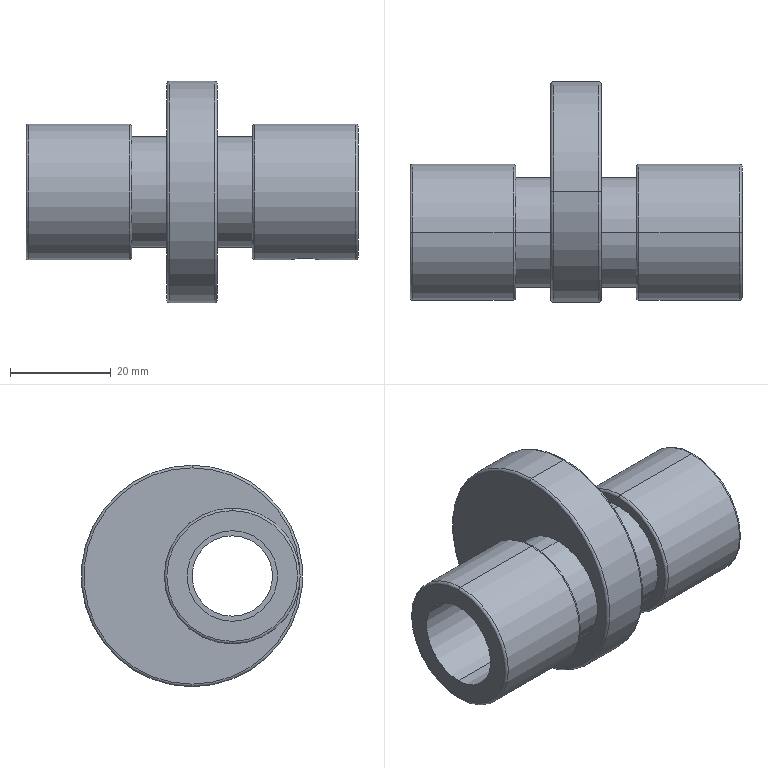Part | SolidWorks | features ICE 3, Fillet 1, Revolution 1 | 1 solid | 38 faces | box 66 x 44 x 44 mm | volume 29541 mm3 | cylinder 18 | torus 12 | plane 8 | commonest cylinder face diameters 18 x4 22 x4 27 x4 6 x2 16 x2 44 x2
STEP:
#1=CARTESIAN_POINT('',(52.5,0.,-13.5));
#2=VERTEX_POINT('',#1);
#3=CARTESIAN_POINT('',(58.5,0.,-13.5));
#4=VERTEX_POINT('',#3);
#5=CARTESIAN_POINT('',(52.5,0.,-13.5));
#6=CARTESIAN_POINT('',(52.5,-0.3922,-13.5));
#7=CARTESIAN_POINT('',(52.579,-0.7881,-13.482));
#8=CARTESIAN_POINT('',(52.804,-1.33,-13.436));
#9=CARTESIAN_POINT('',(52.898,-1.505,-13.417));
#10=CARTESIAN_POINT('',(53.116,-1.831,-13.376));
#11=CARTESIAN_POINT('',(53.239,-1.982,-13.354));
#12=CARTESIAN_POINT('',(53.516,-2.259,-13.31));
#13=CARTESIAN_POINT('',(53.67,-2.385,-13.288));
#14=CARTESIAN_POINT('',(53.994,-2.602,-13.247));
#15=CARTESIAN_POINT('',(54.166,-2.694,-13.229));
#16=CARTESIAN_POINT('',(54.712,-2.922,-13.181));
#17=CARTESIAN_POINT('',(55.103,-3.,-13.162));
#18=CARTESIAN_POINT('',(55.697,-3.,-13.162));
#19=CARTESIAN_POINT('',(55.892,-2.981,-13.167));
#20=CARTESIAN_POINT('',(56.277,-2.904,-13.184));
#21=CARTESIAN_POINT('',(56.468,-2.846,-13.197));
#22=CARTESIAN_POINT('',(56.83,-2.696,-13.228));
#23=CARTESIAN_POINT('',(57.002,-2.604,-13.247));
#24=CARTESIAN_POINT('',(57.329,-2.386,-13.288));
#25=CARTESIAN_POINT('',(57.482,-2.26,-13.31));
#26=CARTESIAN_POINT('',(57.758,-1.985,-13.354));
#27=CARTESIAN_POINT('',(57.883,-1.834,-13.376));
#28=CARTESIAN_POINT('',(58.102,-1.506,-13.417));
#29=CARTESIAN_POINT('',(58.194,-1.333,-13.435));
#30=CARTESIAN_POINT('',(58.345,-0.9726,-13.466));
#31=CARTESIAN_POINT('',(58.403,-0.7819,-13.479));
#32=CARTESIAN_POINT('',(58.48,-0.395,-13.496));
#33=CARTESIAN_POINT('',(58.5,-0.1988,-13.5));
#34=CARTESIAN_POINT('',(58.5,0.,-13.5));
#35=B_SPLINE_CURVE_WITH_KNOTS('',3,(#5,#6,#7,#8,#9,#10,#11,#12,#13,#14,#15,#16,#17,#18,#19,#20,#21,#22,#23,#24,#25,#26,#27,#28,#29,#30,#31,#32,#33,#34),.UNSPECIFIED.,.F.,.F.,(4,2,2,2,2,2,2,2,2,2,2,2,2,2,4),(0.009409,0.01058,0.01117,0.01176,0.01235,0.01294,0.01411,0.0147,0.01529,0.01588,0.01646,0.01705,0.01764,0.01823,0.01882),.UNSPECIFIED.);
#36=EDGE_CURVE('',#2,#4,#35,.T.);
#37=ORIENTED_EDGE('',*,*,#36,.F.);
#38=CARTESIAN_POINT('',(52.5,0.,-9.));
#39=VERTEX_POINT('',#38);
#40=CARTESIAN_POINT('',(52.5,0.,-26.));
#41=DIRECTION('',(0.,0.,1.));
#42=VECTOR('',#41,1000.);
#43=LINE('',#40,#42);
#44=EDGE_CURVE('',#2,#39,#43,.T.);
#45=ORIENTED_EDGE('',*,*,#44,.T.);
#46=CARTESIAN_POINT('',(58.5,0.,-9.));
#47=VERTEX_POINT('',#46);
#48=CARTESIAN_POINT('',(58.5,0.,-9.));
#49=CARTESIAN_POINT('',(58.5,-0.1998,-9.));
#50=CARTESIAN_POINT('',(58.48,-0.3959,-8.993));
#51=CARTESIAN_POINT('',(58.403,-0.7814,-8.968));
#52=CARTESIAN_POINT('',(58.345,-0.9727,-8.949));
#53=CARTESIAN_POINT('',(58.194,-1.335,-8.902));
#54=CARTESIAN_POINT('',(58.101,-1.507,-8.874));
#55=CARTESIAN_POINT('',(57.883,-1.832,-8.813));
#56=CARTESIAN_POINT('',(57.758,-1.985,-8.78));
#57=CARTESIAN_POINT('',(57.346,-2.397,-8.68));
#58=CARTESIAN_POINT('',(57.013,-2.62,-8.612));
#59=CARTESIAN_POINT('',(56.473,-2.845,-8.539));
#60=CARTESIAN_POINT('',(56.282,-2.903,-8.519));
#61=CARTESIAN_POINT('',(55.894,-2.981,-8.492));
#62=CARTESIAN_POINT('',(55.699,-3.,-8.485));
#63=CARTESIAN_POINT('',(55.304,-3.,-8.485));
#64=CARTESIAN_POINT('',(55.104,-2.98,-8.492));
#65=CARTESIAN_POINT('',(54.718,-2.903,-8.519));
#66=CARTESIAN_POINT('',(54.53,-2.846,-8.539));
#67=CARTESIAN_POINT('',(54.165,-2.694,-8.588));
#68=CARTESIAN_POINT('',(53.992,-2.601,-8.617));
#69=CARTESIAN_POINT('',(53.669,-2.384,-8.679));
#70=CARTESIAN_POINT('',(53.516,-2.259,-8.713));
#71=CARTESIAN_POINT('',(53.24,-1.982,-8.78));
#72=CARTESIAN_POINT('',(53.117,-1.832,-8.813));
#73=CARTESIAN_POINT('',(52.899,-1.508,-8.874));
#74=CARTESIAN_POINT('',(52.805,-1.333,-8.903));
#75=CARTESIAN_POINT('',(52.655,-0.9714,-8.949));
#76=CARTESIAN_POINT('',(52.598,-0.7841,-8.968));
#77=CARTESIAN_POINT('',(52.52,-0.3957,-8.993));
#78=CARTESIAN_POINT('',(52.5,-0.1968,-9.));
#79=CARTESIAN_POINT('',(52.5,0.,-9.));
#80=B_SPLINE_CURVE_WITH_KNOTS('',3,(#48,#49,#50,#51,#52,#53,#54,#55,#56,#57,#58,#59,#60,#61,#62,#63,#64,#65,#66,#67,#68,#69,#70,#71,#72,#73,#74,#75,#76,#77,#78,#79),.UNSPECIFIED.,.F.,.F.,(4,2,2,2,2,2,2,2,2,2,2,2,2,2,2,4),(0.,0.0005905,0.001181,0.001771,0.002362,0.003543,0.004133,0.004724,0.005314,0.005905,0.006495,0.007086,0.007676,0.008267,0.008857,0.009447),.UNSPECIFIED.);
#81=EDGE_CURVE('',#47,#39,#80,.T.);
#82=ORIENTED_EDGE('',*,*,#81,.F.);
#83=CARTESIAN_POINT('',(58.5,0.,-26.));
#84=DIRECTION('',(0.,0.,1.));
#85=VECTOR('',#84,1000.);
#86=LINE('',#83,#85);
#87=EDGE_CURVE('',#4,#47,#86,.T.);
#88=ORIENTED_EDGE('',*,*,#87,.F.);
#89=EDGE_LOOP('',(#37,#45,#82,#88));
#90=FACE_OUTER_BOUND('',#89,.T.);
#91=CARTESIAN_POINT('',(55.5,0.,-26.));
#92=DIRECTION('',(0.,0.,1.));
#93=DIRECTION('',(1.,0.,0.));
#94=AXIS2_PLACEMENT_3D('',#91,#92,#93);
#95=CYLINDRICAL_SURFACE('',#94,3.);
#96=ADVANCED_FACE('',(#90),#95,.F.);
#97=CARTESIAN_POINT('',(0.,0.,13.));
#98=VERTEX_POINT('',#97);
#99=CARTESIAN_POINT('',(0.,0.,-13.));
#100=VERTEX_POINT('',#99);
#101=CARTESIAN_POINT('',(0.,0.,0.));
#102=DIRECTION('',(-1.,0.,0.));
#103=DIRECTION('',(0.,0.,-1.));
#104=AXIS2_PLACEMENT_3D('',#101,#102,#103);
#105=CIRCLE('',#104,13.);
#106=EDGE_CURVE('',#98,#100,#105,.T.);
#107=ORIENTED_EDGE('',*,*,#106,.F.);
#108=CARTESIAN_POINT('',(0.5,0.,13.5));
#109=VERTEX_POINT('',#108);
#110=CARTESIAN_POINT('',(0.5,0.,13.));
#111=DIRECTION('',(0.,1.,0.));
#112=DIRECTION('',(0.,0.,1.));
#113=AXIS2_PLACEMENT_3D('',#110,#111,#112);
#114=CIRCLE('',#113,0.5);
#115=EDGE_CURVE('',#98,#109,#114,.T.);
#116=ORIENTED_EDGE('',*,*,#115,.T.);
#117=CARTESIAN_POINT('',(0.5,0.,-13.5));
#118=VERTEX_POINT('',#117);
#119=CARTESIAN_POINT('',(0.5,0.,0.));
#120=DIRECTION('',(1.,0.,0.));
#121=DIRECTION('',(0.,0.,-1.));
#122=AXIS2_PLACEMENT_3D('',#119,#120,#121);
#123=CIRCLE('',#122,13.5);
#124=EDGE_CURVE('',#118,#109,#123,.T.);
#125=ORIENTED_EDGE('',*,*,#124,.F.);
#126=CARTESIAN_POINT('',(0.5,0.,-13.));
#127=DIRECTION('',(0.,-1.,0.));
#128=DIRECTION('',(0.,0.,-1.));
#129=AXIS2_PLACEMENT_3D('',#126,#127,#128);
#130=CIRCLE('',#129,0.5);
#131=EDGE_CURVE('',#100,#118,#130,.T.);
#132=ORIENTED_EDGE('',*,*,#131,.F.);
#133=EDGE_LOOP('',(#107,#116,#125,#132));
#134=FACE_OUTER_BOUND('',#133,.T.);
#135=CARTESIAN_POINT('',(0.5,0.,0.));
#136=DIRECTION('',(1.,0.,0.));
#137=DIRECTION('',(0.,0.,-1.));
#138=AXIS2_PLACEMENT_3D('',#135,#136,#137);
#139=TOROIDAL_SURFACE('',#138,13.,0.5);
#140=ADVANCED_FACE('',(#134),#139,.T.);
#141=CARTESIAN_POINT('',(21.,0.,-13.));
#142=VERTEX_POINT('',#141);
#143=CARTESIAN_POINT('',(21.,0.,13.));
#144=VERTEX_POINT('',#143);
#145=CARTESIAN_POINT('',(21.,0.,0.));
#146=DIRECTION('',(1.,0.,0.));
#147=DIRECTION('',(0.,0.,1.));
#148=AXIS2_PLACEMENT_3D('',#145,#146,#147);
#149=CIRCLE('',#148,13.);
#150=EDGE_CURVE('',#142,#144,#149,.T.);
#151=ORIENTED_EDGE('',*,*,#150,.F.);
#152=CARTESIAN_POINT('',(20.5,0.,-13.5));
#153=VERTEX_POINT('',#152);
#154=CARTESIAN_POINT('',(20.5,0.,-13.));
#155=DIRECTION('',(0.,1.,0.));
#156=DIRECTION('',(0.,0.,1.));
#157=AXIS2_PLACEMENT_3D('',#154,#155,#156);
#158=CIRCLE('',#157,0.5);
#159=EDGE_CURVE('',#142,#153,#158,.T.);
#160=ORIENTED_EDGE('',*,*,#159,.T.);
#161=CARTESIAN_POINT('',(20.5,0.,13.5));
#162=VERTEX_POINT('',#161);
#163=CARTESIAN_POINT('',(20.5,0.,0.));
#164=DIRECTION('',(-1.,0.,0.));
#165=DIRECTION('',(0.,0.,1.));
#166=AXIS2_PLACEMENT_3D('',#163,#164,#165);
#167=CIRCLE('',#166,13.5);
#168=EDGE_CURVE('',#162,#153,#167,.T.);
#169=ORIENTED_EDGE('',*,*,#168,.F.);
#170=CARTESIAN_POINT('',(20.5,0.,13.));
#171=DIRECTION('',(0.,-1.,0.));
#172=DIRECTION('',(0.,0.,-1.));
#173=AXIS2_PLACEMENT_3D('',#170,#171,#172);
#174=CIRCLE('',#173,0.5);
#175=EDGE_CURVE('',#144,#162,#174,.T.);
#176=ORIENTED_EDGE('',*,*,#175,.F.);
#177=EDGE_LOOP('',(#151,#160,#169,#176));
#178=FACE_OUTER_BOUND('',#177,.T.);
#179=CARTESIAN_POINT('',(20.5,0.,0.));
#180=DIRECTION('',(-1.,0.,0.));
#181=DIRECTION('',(0.,0.,1.));
#182=AXIS2_PLACEMENT_3D('',#179,#180,#181);
#183=TOROIDAL_SURFACE('',#182,13.,0.5);
#184=ADVANCED_FACE('',(#178),#183,.T.);
#185=CARTESIAN_POINT('',(38.,8.,-21.5));
#186=VERTEX_POINT('',#185);
#187=CARTESIAN_POINT('',(38.,8.,21.5));
#188=VERTEX_POINT('',#187);
#189=CARTESIAN_POINT('',(38.,8.,0.));
#190=DIRECTION('',(1.,0.,0.));
#191=DIRECTION('',(0.,0.,1.));
#192=AXIS2_PLACEMENT_3D('',#189,#190,#191);
#193=CIRCLE('',#192,21.5);
#194=EDGE_CURVE('',#186,#188,#193,.T.);
#195=ORIENTED_EDGE('',*,*,#194,.F.);
#196=CARTESIAN_POINT('',(37.5,8.,-22.));
#197=VERTEX_POINT('',#196);
#198=CARTESIAN_POINT('',(37.5,8.,-21.5));
#199=DIRECTION('',(0.,1.,0.));
#200=DIRECTION('',(0.,0.,1.));
#201=AXIS2_PLACEMENT_3D('',#198,#199,#200);
#202=CIRCLE('',#201,0.5);
#203=EDGE_CURVE('',#186,#197,#202,.T.);
#204=ORIENTED_EDGE('',*,*,#203,.T.);
#205=CARTESIAN_POINT('',(37.5,8.,22.));
#206=VERTEX_POINT('',#205);
#207=CARTESIAN_POINT('',(37.5,8.,0.));
#208=DIRECTION('',(-1.,0.,0.));
#209=DIRECTION('',(0.,0.,1.));
#210=AXIS2_PLACEMENT_3D('',#207,#208,#209);
#211=CIRCLE('',#210,22.);
#212=EDGE_CURVE('',#206,#197,#211,.T.);
#213=ORIENTED_EDGE('',*,*,#212,.F.);
#214=CARTESIAN_POINT('',(37.5,8.,21.5));
#215=DIRECTION('',(0.,-1.,0.));
#216=DIRECTION('',(0.,0.,-1.));
#217=AXIS2_PLACEMENT_3D('',#214,#215,#216);
#218=CIRCLE('',#217,0.5);
#219=EDGE_CURVE('',#188,#206,#218,.T.);
#220=ORIENTED_EDGE('',*,*,#219,.F.);
#221=EDGE_LOOP('',(#195,#204,#213,#220));
#222=FACE_OUTER_BOUND('',#221,.T.);
#223=CARTESIAN_POINT('',(37.5,8.,0.));
#224=DIRECTION('',(-1.,0.,0.));
#225=DIRECTION('',(0.,0.,1.));
#226=AXIS2_PLACEMENT_3D('',#223,#224,#225);
#227=TOROIDAL_SURFACE('',#226,21.5,0.5);
#228=ADVANCED_FACE('',(#222),#227,.T.);
#229=CARTESIAN_POINT('',(28.5,8.,-22.));
#230=VERTEX_POINT('',#229);
#231=CARTESIAN_POINT('',(28.5,8.,22.));
#232=VERTEX_POINT('',#231);
#233=CARTESIAN_POINT('',(28.5,8.,0.));
#234=DIRECTION('',(1.,0.,0.));
#235=DIRECTION('',(0.,0.,1.));
#236=AXIS2_PLACEMENT_3D('',#233,#234,#235);
#237=CIRCLE('',#236,22.);
#238=EDGE_CURVE('',#230,#232,#237,.T.);
#239=ORIENTED_EDGE('',*,*,#238,.F.);
#240=CARTESIAN_POINT('',(28.,8.,-21.5));
#241=VERTEX_POINT('',#240);
#242=CARTESIAN_POINT('',(28.5,8.,-21.5));
#243=DIRECTION('',(0.,1.,0.));
#244=DIRECTION('',(0.,0.,1.));
#245=AXIS2_PLACEMENT_3D('',#242,#243,#244);
#246=CIRCLE('',#245,0.5);
#247=EDGE_CURVE('',#230,#241,#246,.T.);
#248=ORIENTED_EDGE('',*,*,#247,.T.);
#249=CARTESIAN_POINT('',(28.,8.,21.5));
#250=VERTEX_POINT('',#249);
#251=CARTESIAN_POINT('',(28.,8.,0.));
#252=DIRECTION('',(-1.,0.,0.));
#253=DIRECTION('',(0.,0.,1.));
#254=AXIS2_PLACEMENT_3D('',#251,#252,#253);
#255=CIRCLE('',#254,21.5);
#256=EDGE_CURVE('',#250,#241,#255,.T.);
#257=ORIENTED_EDGE('',*,*,#256,.F.);
#258=CARTESIAN_POINT('',(28.5,8.,21.5));
#259=DIRECTION('',(0.,-1.,0.));
#260=DIRECTION('',(0.,0.,-1.));
#261=AXIS2_PLACEMENT_3D('',#258,#259,#260);
#262=CIRCLE('',#261,0.5);
#263=EDGE_CURVE('',#232,#250,#262,.T.);
#264=ORIENTED_EDGE('',*,*,#263,.F.);
#265=EDGE_LOOP('',(#239,#248,#257,#264));
#266=FACE_OUTER_BOUND('',#265,.T.);
#267=CARTESIAN_POINT('',(28.5,8.,0.));
#268=DIRECTION('',(-1.,0.,0.));
#269=DIRECTION('',(0.,0.,1.));
#270=AXIS2_PLACEMENT_3D('',#267,#268,#269);
#271=TOROIDAL_SURFACE('',#270,21.5,0.5);
#272=ADVANCED_FACE('',(#266),#271,.T.);
#273=CARTESIAN_POINT('',(45.,0.,13.));
#274=VERTEX_POINT('',#273);
#275=CARTESIAN_POINT('',(45.,0.,-13.));
#276=VERTEX_POINT('',#275);
#277=CARTESIAN_POINT('',(45.,0.,0.));
#278=DIRECTION('',(-1.,0.,0.));
#279=DIRECTION('',(0.,0.,-1.));
#280=AXIS2_PLACEMENT_3D('',#277,#278,#279);
#281=CIRCLE('',#280,13.);
#282=EDGE_CURVE('',#274,#276,#281,.T.);
#283=ORIENTED_EDGE('',*,*,#282,.F.);
#284=CARTESIAN_POINT('',(45.5,0.,13.5));
#285=VERTEX_POINT('',#284);
#286=CARTESIAN_POINT('',(45.5,0.,13.));
#287=DIRECTION('',(0.,1.,0.));
#288=DIRECTION('',(0.,0.,1.));
#289=AXIS2_PLACEMENT_3D('',#286,#287,#288);
#290=CIRCLE('',#289,0.5);
#291=EDGE_CURVE('',#274,#285,#290,.T.);
#292=ORIENTED_EDGE('',*,*,#291,.T.);
#293=CARTESIAN_POINT('',(45.5,0.,-13.5));
#294=VERTEX_POINT('',#293);
#295=CARTESIAN_POINT('',(45.5,0.,0.));
#296=DIRECTION('',(1.,0.,0.));
#297=DIRECTION('',(0.,0.,-1.));
#298=AXIS2_PLACEMENT_3D('',#295,#296,#297);
#299=CIRCLE('',#298,13.5);
#300=EDGE_CURVE('',#294,#285,#299,.T.);
#301=ORIENTED_EDGE('',*,*,#300,.F.);
#302=CARTESIAN_POINT('',(45.5,0.,-13.));
#303=DIRECTION('',(0.,-1.,0.));
#304=DIRECTION('',(0.,0.,-1.));
#305=AXIS2_PLACEMENT_3D('',#302,#303,#304);
#306=CIRCLE('',#305,0.5);
#307=EDGE_CURVE('',#276,#294,#306,.T.);
#308=ORIENTED_EDGE('',*,*,#307,.F.);
#309=EDGE_LOOP('',(#283,#292,#301,#308));
#310=FACE_OUTER_BOUND('',#309,.T.);
#311=CARTESIAN_POINT('',(45.5,0.,0.));
#312=DIRECTION('',(1.,0.,0.));
#313=DIRECTION('',(0.,0.,-1.));
#314=AXIS2_PLACEMENT_3D('',#311,#312,#313);
#315=TOROIDAL_SURFACE('',#314,13.,0.5);
#316=ADVANCED_FACE('',(#310),#315,.T.);
#317=CARTESIAN_POINT('',(66.,0.,-13.));
#318=VERTEX_POINT('',#317);
#319=CARTESIAN_POINT('',(66.,0.,13.));
#320=VERTEX_POINT('',#319);
#321=CARTESIAN_POINT('',(66.,0.,0.));
#322=DIRECTION('',(1.,0.,0.));
#323=DIRECTION('',(0.,0.,1.));
#324=AXIS2_PLACEMENT_3D('',#321,#322,#323);
#325=CIRCLE('',#324,13.);
#326=EDGE_CURVE('',#318,#320,#325,.T.);
#327=ORIENTED_EDGE('',*,*,#326,.F.);
#328=CARTESIAN_POINT('',(65.5,0.,-13.5));
#329=VERTEX_POINT('',#328);
#330=CARTESIAN_POINT('',(65.5,0.,-13.));
#331=DIRECTION('',(0.,1.,0.));
#332=DIRECTION('',(0.,0.,1.));
#333=AXIS2_PLACEMENT_3D('',#330,#331,#332);
#334=CIRCLE('',#333,0.5);
#335=EDGE_CURVE('',#318,#329,#334,.T.);
#336=ORIENTED_EDGE('',*,*,#335,.T.);
#337=CARTESIAN_POINT('',(65.5,0.,13.5));
#338=VERTEX_POINT('',#337);
#339=CARTESIAN_POINT('',(65.5,0.,0.));
#340=DIRECTION('',(-1.,0.,0.));
#341=DIRECTION('',(0.,0.,1.));
#342=AXIS2_PLACEMENT_3D('',#339,#340,#341);
#343=CIRCLE('',#342,13.5);
#344=EDGE_CURVE('',#338,#329,#343,.T.);
#345=ORIENTED_EDGE('',*,*,#344,.F.);
#346=CARTESIAN_POINT('',(65.5,0.,13.));
#347=DIRECTION('',(0.,-1.,0.));
#348=DIRECTION('',(0.,0.,-1.));
#349=AXIS2_PLACEMENT_3D('',#346,#347,#348);
#350=CIRCLE('',#349,0.5);
#351=EDGE_CURVE('',#320,#338,#350,.T.);
#352=ORIENTED_EDGE('',*,*,#351,.F.);
#353=EDGE_LOOP('',(#327,#336,#345,#352));
#354=FACE_OUTER_BOUND('',#353,.T.);
#355=CARTESIAN_POINT('',(65.5,0.,0.));
#356=DIRECTION('',(-1.,0.,0.));
#357=DIRECTION('',(0.,0.,1.));
#358=AXIS2_PLACEMENT_3D('',#355,#356,#357);
#359=TOROIDAL_SURFACE('',#358,13.,0.5);
#360=ADVANCED_FACE('',(#354),#359,.T.);
#361=CARTESIAN_POINT('',(51.,0.,-8.));
#362=VERTEX_POINT('',#361);
#363=CARTESIAN_POINT('',(51.,0.,8.));
#364=VERTEX_POINT('',#363);
#365=CARTESIAN_POINT('',(51.,0.,0.));
#366=DIRECTION('',(-1.,0.,0.));
#367=DIRECTION('',(0.,0.,1.));
#368=AXIS2_PLACEMENT_3D('',#365,#366,#367);
#369=CIRCLE('',#368,8.);
#370=EDGE_CURVE('',#362,#364,#369,.T.);
#371=ORIENTED_EDGE('',*,*,#370,.F.);
#372=CARTESIAN_POINT('',(15.,0.,-8.));
#373=VERTEX_POINT('',#372);
#374=CARTESIAN_POINT('',(0.,0.,-8.));
#375=DIRECTION('',(-1.,0.,0.));
#376=VECTOR('',#375,1000.);
#377=LINE('',#374,#376);
#378=EDGE_CURVE('',#362,#373,#377,.T.);
#379=ORIENTED_EDGE('',*,*,#378,.T.);
#380=CARTESIAN_POINT('',(15.,0.,8.));
#381=VERTEX_POINT('',#380);
#382=CARTESIAN_POINT('',(15.,0.,0.));
#383=DIRECTION('',(-1.,0.,0.));
#384=DIRECTION('',(0.,0.,1.));
#385=AXIS2_PLACEMENT_3D('',#382,#383,#384);
#386=CIRCLE('',#385,8.);
#387=EDGE_CURVE('',#373,#381,#386,.T.);
#388=ORIENTED_EDGE('',*,*,#387,.T.);
#389=CARTESIAN_POINT('',(0.,0.,8.));
#390=DIRECTION('',(-1.,0.,0.));
#391=VECTOR('',#390,1000.);
#392=LINE('',#389,#391);
#393=EDGE_CURVE('',#364,#381,#392,.T.);
#394=ORIENTED_EDGE('',*,*,#393,.F.);
#395=EDGE_LOOP('',(#371,#379,#388,#394));
#396=FACE_OUTER_BOUND('',#395,.T.);
#397=CARTESIAN_POINT('',(0.,0.,0.));
#398=DIRECTION('',(-1.,0.,0.));
#399=DIRECTION('',(0.,0.,1.));
#400=AXIS2_PLACEMENT_3D('',#397,#398,#399);
#401=CYLINDRICAL_SURFACE('',#400,8.);
#402=ADVANCED_FACE('',(#396),#401,.F.);
#403=CARTESIAN_POINT('',(15.,0.,-9.));
#404=VERTEX_POINT('',#403);
#405=CARTESIAN_POINT('',(15.,0.,9.));
#406=VERTEX_POINT('',#405);
#407=CARTESIAN_POINT('',(15.,0.,0.));
#408=DIRECTION('',(-1.,0.,0.));
#409=DIRECTION('',(0.,0.,1.));
#410=AXIS2_PLACEMENT_3D('',#407,#408,#409);
#411=CIRCLE('',#410,9.);
#412=EDGE_CURVE('',#404,#406,#411,.T.);
#413=ORIENTED_EDGE('',*,*,#412,.F.);
#414=CARTESIAN_POINT('',(0.,0.,-9.));
#415=VERTEX_POINT('',#414);
#416=CARTESIAN_POINT('',(0.,0.,-9.));
#417=DIRECTION('',(-1.,0.,0.));
#418=VECTOR('',#417,1000.);
#419=LINE('',#416,#418);
#420=EDGE_CURVE('',#404,#415,#419,.T.);
#421=ORIENTED_EDGE('',*,*,#420,.T.);
#422=CARTESIAN_POINT('',(0.,0.,9.));
#423=VERTEX_POINT('',#422);
#424=CARTESIAN_POINT('',(0.,0.,0.));
#425=DIRECTION('',(-1.,0.,0.));
#426=DIRECTION('',(0.,0.,1.));
#427=AXIS2_PLACEMENT_3D('',#424,#425,#426);
#428=CIRCLE('',#427,9.);
#429=EDGE_CURVE('',#415,#423,#428,.T.);
#430=ORIENTED_EDGE('',*,*,#429,.T.);
#431=CARTESIAN_POINT('',(0.,0.,9.));
#432=DIRECTION('',(-1.,0.,0.));
#433=VECTOR('',#432,1000.);
#434=LINE('',#431,#433);
#435=EDGE_CURVE('',#406,#423,#434,.T.);
#436=ORIENTED_EDGE('',*,*,#435,.F.);
#437=EDGE_LOOP('',(#413,#421,#430,#436));
#438=FACE_OUTER_BOUND('',#437,.T.);
#439=CARTESIAN_POINT('',(0.,0.,0.));
#440=DIRECTION('',(-1.,0.,0.));
#441=DIRECTION('',(0.,0.,1.));
#442=AXIS2_PLACEMENT_3D('',#439,#440,#441);
#443=CYLINDRICAL_SURFACE('',#442,9.);
#444=ADVANCED_FACE('',(#438),#443,.F.);
#445=CARTESIAN_POINT('',(28.,0.,11.));
#446=VERTEX_POINT('',#445);
#447=CARTESIAN_POINT('',(28.,0.,-11.));
#448=VERTEX_POINT('',#447);
#449=CARTESIAN_POINT('',(28.,0.,0.));
#450=DIRECTION('',(-1.,0.,0.));
#451=DIRECTION('',(0.,0.,1.));
#452=AXIS2_PLACEMENT_3D('',#449,#450,#451);
#453=CIRCLE('',#452,11.);
#454=EDGE_CURVE('',#446,#448,#453,.T.);
#455=ORIENTED_EDGE('',*,*,#454,.T.);
#456=CARTESIAN_POINT('',(21.,0.,-11.));
#457=VERTEX_POINT('',#456);
#458=CARTESIAN_POINT('',(0.,0.,-11.));
#459=DIRECTION('',(-1.,0.,0.));
#460=VECTOR('',#459,1000.);
#461=LINE('',#458,#460);
#462=EDGE_CURVE('',#448,#457,#461,.T.);
#463=ORIENTED_EDGE('',*,*,#462,.T.);
#464=CARTESIAN_POINT('',(21.,0.,11.));
#465=VERTEX_POINT('',#464);
#466=CARTESIAN_POINT('',(21.,0.,0.));
#467=DIRECTION('',(-1.,0.,0.));
#468=DIRECTION('',(0.,0.,1.));
#469=AXIS2_PLACEMENT_3D('',#466,#467,#468);
#470=CIRCLE('',#469,11.);
#471=EDGE_CURVE('',#465,#457,#470,.T.);
#472=ORIENTED_EDGE('',*,*,#471,.F.);
#473=CARTESIAN_POINT('',(0.,0.,11.));
#474=DIRECTION('',(-1.,0.,0.));
#475=VECTOR('',#474,1000.);
#476=LINE('',#473,#475);
#477=EDGE_CURVE('',#446,#465,#476,.T.);
#478=ORIENTED_EDGE('',*,*,#477,.F.);
#479=EDGE_LOOP('',(#455,#463,#472,#478));
#480=FACE_OUTER_BOUND('',#479,.T.);
#481=CARTESIAN_POINT('',(0.,0.,0.));
#482=DIRECTION('',(-1.,0.,0.));
#483=DIRECTION('',(0.,0.,1.));
#484=AXIS2_PLACEMENT_3D('',#481,#482,#483);
#485=CYLINDRICAL_SURFACE('',#484,11.);
#486=ADVANCED_FACE('',(#480),#485,.T.);
#487=ORIENTED_EDGE('',*,*,#168,.T.);
#488=CARTESIAN_POINT('',(0.,0.,-13.5));
#489=DIRECTION('',(-1.,0.,0.));
#490=VECTOR('',#489,1000.);
#491=LINE('',#488,#490);
#492=EDGE_CURVE('',#153,#118,#491,.T.);
#493=ORIENTED_EDGE('',*,*,#492,.T.);
#494=ORIENTED_EDGE('',*,*,#124,.T.);
#495=CARTESIAN_POINT('',(0.,0.,13.5));
#496=DIRECTION('',(-1.,0.,0.));
#497=VECTOR('',#496,1000.);
#498=LINE('',#495,#497);
#499=EDGE_CURVE('',#162,#109,#498,.T.);
#500=ORIENTED_EDGE('',*,*,#499,.F.);
#501=EDGE_LOOP('',(#487,#493,#494,#500));
#502=FACE_OUTER_BOUND('',#501,.T.);
#503=CARTESIAN_POINT('',(0.,0.,0.));
#504=DIRECTION('',(-1.,0.,0.));
#505=DIRECTION('',(0.,0.,1.));
#506=AXIS2_PLACEMENT_3D('',#503,#504,#505);
#507=CYLINDRICAL_SURFACE('',#506,13.5);
#508=ADVANCED_FACE('',(#502),#507,.T.);
#509=ORIENTED_EDGE('',*,*,#212,.T.);
#510=CARTESIAN_POINT('',(38.,8.,-22.));
#511=DIRECTION('',(-1.,0.,0.));
#512=VECTOR('',#511,1000.);
#513=LINE('',#510,#512);
#514=EDGE_CURVE('',#197,#230,#513,.T.);
#515=ORIENTED_EDGE('',*,*,#514,.T.);
#516=ORIENTED_EDGE('',*,*,#238,.T.);
#517=CARTESIAN_POINT('',(38.,8.,22.));
#518=DIRECTION('',(-1.,0.,0.));
#519=VECTOR('',#518,1000.);
#520=LINE('',#517,#519);
#521=EDGE_CURVE('',#206,#232,#520,.T.);
#522=ORIENTED_EDGE('',*,*,#521,.F.);
#523=EDGE_LOOP('',(#509,#515,#516,#522));
#524=FACE_OUTER_BOUND('',#523,.T.);
#525=CARTESIAN_POINT('',(38.,8.,0.));
#526=DIRECTION('',(-1.,0.,0.));
#527=DIRECTION('',(0.,0.,1.));
#528=AXIS2_PLACEMENT_3D('',#525,#526,#527);
#529=CYLINDRICAL_SURFACE('',#528,22.);
#530=ADVANCED_FACE('',(#524),#529,.T.);
#531=CARTESIAN_POINT('',(66.,0.,-9.));
#532=VERTEX_POINT('',#531);
#533=CARTESIAN_POINT('',(66.,0.,9.));
#534=VERTEX_POINT('',#533);
#535=CARTESIAN_POINT('',(66.,0.,0.));
#536=DIRECTION('',(-1.,0.,0.));
#537=DIRECTION('',(0.,0.,1.));
#538=AXIS2_PLACEMENT_3D('',#535,#536,#537);
#539=CIRCLE('',#538,9.);
#540=EDGE_CURVE('',#532,#534,#539,.T.);
#541=ORIENTED_EDGE('',*,*,#540,.F.);
#542=CARTESIAN_POINT('',(0.,0.,-9.));
#543=DIRECTION('',(-1.,0.,0.));
#544=VECTOR('',#543,1000.);
#545=LINE('',#542,#544);
#546=EDGE_CURVE('',#532,#47,#545,.T.);
#547=ORIENTED_EDGE('',*,*,#546,.T.);
#548=ORIENTED_EDGE('',*,*,#81,.T.);
#549=CARTESIAN_POINT('',(51.,0.,-9.));
#550=VERTEX_POINT('',#549);
#551=CARTESIAN_POINT('',(0.,0.,-9.));
#552=DIRECTION('',(-1.,0.,0.));
#553=VECTOR('',#552,1000.);
#554=LINE('',#551,#553);
#555=EDGE_CURVE('',#39,#550,#554,.T.);
#556=ORIENTED_EDGE('',*,*,#555,.T.);
#557=CARTESIAN_POINT('',(51.,0.,9.));
#558=VERTEX_POINT('',#557);
#559=CARTESIAN_POINT('',(51.,0.,0.));
#560=DIRECTION('',(-1.,0.,0.));
#561=DIRECTION('',(0.,0.,1.));
#562=AXIS2_PLACEMENT_3D('',#559,#560,#561);
#563=CIRCLE('',#562,9.);
#564=EDGE_CURVE('',#550,#558,#563,.T.);
#565=ORIENTED_EDGE('',*,*,#564,.T.);
#566=CARTESIAN_POINT('',(0.,0.,9.));
#567=DIRECTION('',(-1.,0.,0.));
#568=VECTOR('',#567,1000.);
#569=LINE('',#566,#568);
#570=EDGE_CURVE('',#534,#558,#569,.T.);
#571=ORIENTED_EDGE('',*,*,#570,.F.);
#572=EDGE_LOOP('',(#541,#547,#548,#556,#565,#571));
#573=FACE_OUTER_BOUND('',#572,.T.);
#574=CARTESIAN_POINT('',(0.,0.,0.));
#575=DIRECTION('',(-1.,0.,0.));
#576=DIRECTION('',(0.,0.,1.));
#577=AXIS2_PLACEMENT_3D('',#574,#575,#576);
#578=CYLINDRICAL_SURFACE('',#577,9.);
#579=ADVANCED_FACE('',(#573),#578,.F.);
#580=ORIENTED_EDGE('',*,*,#344,.T.);
#581=CARTESIAN_POINT('',(0.,0.,-13.5));
#582=DIRECTION('',(-1.,0.,0.));
#583=VECTOR('',#582,1000.);
#584=LINE('',#581,#583);
#585=EDGE_CURVE('',#329,#4,#584,.T.);
#586=ORIENTED_EDGE('',*,*,#585,.T.);
#587=CARTESIAN_POINT('',(58.5,0.,-13.5));
#588=CARTESIAN_POINT('',(58.5,0.1989,-13.5));
#589=CARTESIAN_POINT('',(58.48,0.3943,-13.496));
#590=CARTESIAN_POINT('',(58.404,0.7786,-13.479));
#591=CARTESIAN_POINT('',(58.346,0.9695,-13.466));
#592=CARTESIAN_POINT('',(58.195,1.333,-13.435));
#593=CARTESIAN_POINT('',(58.103,1.505,-13.417));
#594=CARTESIAN_POINT('',(57.885,1.83,-13.376));
#595=CARTESIAN_POINT('',(57.759,1.984,-13.354));
#596=CARTESIAN_POINT('',(57.483,2.26,-13.31));
#597=CARTESIAN_POINT('',(57.332,2.384,-13.288));
#598=CARTESIAN_POINT('',(57.004,2.603,-13.247));
#599=CARTESIAN_POINT('',(56.831,2.696,-13.228));
#600=CARTESIAN_POINT('',(56.47,2.846,-13.197));
#601=CARTESIAN_POINT('',(56.28,2.903,-13.184));
#602=CARTESIAN_POINT('',(55.893,2.981,-13.167));
#603=CARTESIAN_POINT('',(55.698,3.,-13.162));
#604=CARTESIAN_POINT('',(55.305,3.,-13.162));
#605=CARTESIAN_POINT('',(55.105,2.98,-13.167));
#606=CARTESIAN_POINT('',(54.72,2.903,-13.184));
#607=CARTESIAN_POINT('',(54.533,2.847,-13.197));
#608=CARTESIAN_POINT('',(54.169,2.696,-13.228));
#609=CARTESIAN_POINT('',(53.994,2.602,-13.247));
#610=CARTESIAN_POINT('',(53.67,2.385,-13.288));
#611=CARTESIAN_POINT('',(53.518,2.26,-13.31));
#612=CARTESIAN_POINT('',(53.239,1.982,-13.354));
#613=CARTESIAN_POINT('',(53.116,1.831,-13.376));
#614=CARTESIAN_POINT('',(52.898,1.507,-13.417));
#615=CARTESIAN_POINT('',(52.804,1.331,-13.435));
#616=CARTESIAN_POINT('',(52.654,0.9683,-13.466));
#617=CARTESIAN_POINT('',(52.597,0.7813,-13.479));
#618=CARTESIAN_POINT('',(52.52,0.3953,-13.496));
#619=CARTESIAN_POINT('',(52.5,0.1961,-13.5));
#620=CARTESIAN_POINT('',(52.5,0.,-13.5));
#621=B_SPLINE_CURVE_WITH_KNOTS('',3,(#587,#588,#589,#590,#591,#592,#593,#594,#595,#596,#597,#598,#599,#600,#601,#602,#603,#604,#605,#606,#607,#608,#609,#610,#611,#612,#613,#614,#615,#616,#617,#618,#619,#620),.UNSPECIFIED.,.F.,.F.,(4,2,2,2,2,2,2,2,2,2,2,2,2,2,2,2,4),(0.,0.0005881,0.001176,0.001764,0.002352,0.00294,0.003528,0.004116,0.004704,0.005292,0.005881,0.006469,0.007057,0.007645,0.008233,0.008821,0.009409),.UNSPECIFIED.);
#622=EDGE_CURVE('',#4,#2,#621,.T.);
#623=ORIENTED_EDGE('',*,*,#622,.T.);
#624=CARTESIAN_POINT('',(0.,0.,-13.5));
#625=DIRECTION('',(-1.,0.,0.));
#626=VECTOR('',#625,1000.);
#627=LINE('',#624,#626);
#628=EDGE_CURVE('',#2,#294,#627,.T.);
#629=ORIENTED_EDGE('',*,*,#628,.T.);
#630=ORIENTED_EDGE('',*,*,#300,.T.);
#631=CARTESIAN_POINT('',(0.,0.,13.5));
#632=DIRECTION('',(-1.,0.,0.));
#633=VECTOR('',#632,1000.);
#634=LINE('',#631,#633);
#635=EDGE_CURVE('',#338,#285,#634,.T.);
#636=ORIENTED_EDGE('',*,*,#635,.F.);
#637=EDGE_LOOP('',(#580,#586,#623,#629,#630,#636));
#638=FACE_OUTER_BOUND('',#637,.T.);
#639=CARTESIAN_POINT('',(0.,0.,0.));
#640=DIRECTION('',(-1.,0.,0.));
#641=DIRECTION('',(0.,0.,1.));
#642=AXIS2_PLACEMENT_3D('',#639,#640,#641);
#643=CYLINDRICAL_SURFACE('',#642,13.5);
#644=ADVANCED_FACE('',(#638),#643,.T.);
#645=CARTESIAN_POINT('',(45.,0.,11.));
#646=VERTEX_POINT('',#645);
#647=CARTESIAN_POINT('',(45.,0.,-11.));
#648=VERTEX_POINT('',#647);
#649=CARTESIAN_POINT('',(45.,0.,0.));
#650=DIRECTION('',(-1.,0.,0.));
#651=DIRECTION('',(0.,0.,1.));
#652=AXIS2_PLACEMENT_3D('',#649,#650,#651);
#653=CIRCLE('',#652,11.);
#654=EDGE_CURVE('',#646,#648,#653,.T.);
#655=ORIENTED_EDGE('',*,*,#654,.T.);
#656=CARTESIAN_POINT('',(38.,0.,-11.));
#657=VERTEX_POINT('',#656);
#658=CARTESIAN_POINT('',(0.,0.,-11.));
#659=DIRECTION('',(-1.,0.,0.));
#660=VECTOR('',#659,1000.);
#661=LINE('',#658,#660);
#662=EDGE_CURVE('',#648,#657,#661,.T.);
#663=ORIENTED_EDGE('',*,*,#662,.T.);
#664=CARTESIAN_POINT('',(38.,0.,11.));
#665=VERTEX_POINT('',#664);
#666=CARTESIAN_POINT('',(38.,0.,0.));
#667=DIRECTION('',(-1.,0.,0.));
#668=DIRECTION('',(0.,0.,1.));
#669=AXIS2_PLACEMENT_3D('',#666,#667,#668);
#670=CIRCLE('',#669,11.);
#671=EDGE_CURVE('',#665,#657,#670,.T.);
#672=ORIENTED_EDGE('',*,*,#671,.F.);
#673=CARTESIAN_POINT('',(0.,0.,11.));
#674=DIRECTION('',(-1.,0.,0.));
#675=VECTOR('',#674,1000.);
#676=LINE('',#673,#675);
#677=EDGE_CURVE('',#646,#665,#676,.T.);
#678=ORIENTED_EDGE('',*,*,#677,.F.);
#679=EDGE_LOOP('',(#655,#663,#672,#678));
#680=FACE_OUTER_BOUND('',#679,.T.);
#681=CARTESIAN_POINT('',(0.,0.,0.));
#682=DIRECTION('',(-1.,0.,0.));
#683=DIRECTION('',(0.,0.,1.));
#684=AXIS2_PLACEMENT_3D('',#681,#682,#683);
#685=CYLINDRICAL_SURFACE('',#684,11.);
#686=ADVANCED_FACE('',(#680),#685,.T.);
#687=ORIENTED_EDGE('',*,*,#662,.F.);
#688=CARTESIAN_POINT('',(45.,0.,0.));
#689=DIRECTION('',(-1.,0.,0.));
#690=DIRECTION('',(0.,0.,1.));
#691=AXIS2_PLACEMENT_3D('',#688,#689,#690);
#692=CIRCLE('',#691,11.);
#693=EDGE_CURVE('',#648,#646,#692,.T.);
#694=ORIENTED_EDGE('',*,*,#693,.T.);
#695=ORIENTED_EDGE('',*,*,#677,.T.);
#696=CARTESIAN_POINT('',(38.,0.,0.));
#697=DIRECTION('',(-1.,0.,0.));
#698=DIRECTION('',(0.,0.,1.));
#699=AXIS2_PLACEMENT_3D('',#696,#697,#698);
#700=CIRCLE('',#699,11.);
#701=EDGE_CURVE('',#657,#665,#700,.T.);
#702=ORIENTED_EDGE('',*,*,#701,.F.);
#703=EDGE_LOOP('',(#687,#694,#695,#702));
#704=FACE_OUTER_BOUND('',#703,.T.);
#705=CARTESIAN_POINT('',(0.,0.,0.));
#706=DIRECTION('',(-1.,0.,0.));
#707=DIRECTION('',(0.,0.,1.));
#708=AXIS2_PLACEMENT_3D('',#705,#706,#707);
#709=CYLINDRICAL_SURFACE('',#708,11.);
#710=ADVANCED_FACE('',(#704),#709,.T.);
#711=CARTESIAN_POINT('',(45.,0.,0.));
#712=DIRECTION('',(-1.,0.,0.));
#713=DIRECTION('',(0.,0.,-1.));
#714=AXIS2_PLACEMENT_3D('',#711,#712,#713);
#715=CIRCLE('',#714,13.);
#716=EDGE_CURVE('',#276,#274,#715,.T.);
#717=ORIENTED_EDGE('',*,*,#716,.T.);
#718=ORIENTED_EDGE('',*,*,#282,.T.);
#719=EDGE_LOOP('',(#717,#718));
#720=FACE_OUTER_BOUND('',#719,.T.);
#721=ORIENTED_EDGE('',*,*,#654,.F.);
#722=ORIENTED_EDGE('',*,*,#693,.F.);
#723=EDGE_LOOP('',(#721,#722));
#724=FACE_BOUND('',#723,.T.);
#725=CARTESIAN_POINT('',(45.,11.,0.));
#726=DIRECTION('',(1.,0.,0.));
#727=DIRECTION('',(0.,0.,-1.));
#728=AXIS2_PLACEMENT_3D('',#725,#726,#727);
#729=PLANE('',#728);
#730=ADVANCED_FACE('',(#720,#724),#729,.F.);
#731=ORIENTED_EDGE('',*,*,#585,.F.);
#732=CARTESIAN_POINT('',(65.5,0.,0.));
#733=DIRECTION('',(-1.,0.,0.));
#734=DIRECTION('',(0.,0.,1.));
#735=AXIS2_PLACEMENT_3D('',#732,#733,#734);
#736=CIRCLE('',#735,13.5);
#737=EDGE_CURVE('',#329,#338,#736,.T.);
#738=ORIENTED_EDGE('',*,*,#737,.T.);
#739=ORIENTED_EDGE('',*,*,#635,.T.);
#740=CARTESIAN_POINT('',(45.5,0.,0.));
#741=DIRECTION('',(1.,0.,0.));
#742=DIRECTION('',(0.,0.,-1.));
#743=AXIS2_PLACEMENT_3D('',#740,#741,#742);
#744=CIRCLE('',#743,13.5);
#745=EDGE_CURVE('',#285,#294,#744,.T.);
#746=ORIENTED_EDGE('',*,*,#745,.T.);
#747=ORIENTED_EDGE('',*,*,#628,.F.);
#748=ORIENTED_EDGE('',*,*,#36,.T.);
#749=EDGE_LOOP('',(#731,#738,#739,#746,#747,#748));
#750=FACE_OUTER_BOUND('',#749,.T.);
#751=CARTESIAN_POINT('',(0.,0.,0.));
#752=DIRECTION('',(-1.,0.,0.));
#753=DIRECTION('',(0.,0.,1.));
#754=AXIS2_PLACEMENT_3D('',#751,#752,#753);
#755=CYLINDRICAL_SURFACE('',#754,13.5);
#756=ADVANCED_FACE('',(#750),#755,.T.);
#757=CARTESIAN_POINT('',(66.,0.,0.));
#758=DIRECTION('',(1.,0.,0.));
#759=DIRECTION('',(0.,0.,1.));
#760=AXIS2_PLACEMENT_3D('',#757,#758,#759);
#761=CIRCLE('',#760,13.);
#762=EDGE_CURVE('',#320,#318,#761,.T.);
#763=ORIENTED_EDGE('',*,*,#762,.T.);
#764=ORIENTED_EDGE('',*,*,#326,.T.);
#765=EDGE_LOOP('',(#763,#764));
#766=FACE_OUTER_BOUND('',#765,.T.);
#767=CARTESIAN_POINT('',(66.,0.,0.));
#768=DIRECTION('',(-1.,0.,0.));
#769=DIRECTION('',(0.,0.,1.));
#770=AXIS2_PLACEMENT_3D('',#767,#768,#769);
#771=CIRCLE('',#770,9.);
#772=EDGE_CURVE('',#534,#532,#771,.T.);
#773=ORIENTED_EDGE('',*,*,#772,.T.);
#774=ORIENTED_EDGE('',*,*,#540,.T.);
#775=EDGE_LOOP('',(#773,#774));
#776=FACE_BOUND('',#775,.T.);
#777=CARTESIAN_POINT('',(66.,13.5,0.));
#778=DIRECTION('',(-1.,0.,0.));
#779=DIRECTION('',(0.,0.,1.));
#780=AXIS2_PLACEMENT_3D('',#777,#778,#779);
#781=PLANE('',#780);
#782=ADVANCED_FACE('',(#766,#776),#781,.F.);
#783=ORIENTED_EDGE('',*,*,#546,.F.);
#784=ORIENTED_EDGE('',*,*,#772,.F.);
#785=ORIENTED_EDGE('',*,*,#570,.T.);
#786=CARTESIAN_POINT('',(51.,0.,0.));
#787=DIRECTION('',(-1.,0.,0.));
#788=DIRECTION('',(0.,0.,1.));
#789=AXIS2_PLACEMENT_3D('',#786,#787,#788);
#790=CIRCLE('',#789,9.);
#791=EDGE_CURVE('',#558,#550,#790,.T.);
#792=ORIENTED_EDGE('',*,*,#791,.T.);
#793=ORIENTED_EDGE('',*,*,#555,.F.);
#794=CARTESIAN_POINT('',(52.5,0.,-9.));
#795=CARTESIAN_POINT('',(52.5,0.1967,-9.));
#796=CARTESIAN_POINT('',(52.519,0.3948,-8.993));
#797=CARTESIAN_POINT('',(52.597,0.784,-8.968));
#798=CARTESIAN_POINT('',(52.655,0.9716,-8.949));
#799=CARTESIAN_POINT('',(52.806,1.334,-8.903));
#800=CARTESIAN_POINT('',(52.9,1.509,-8.874));
#801=CARTESIAN_POINT('',(53.117,1.833,-8.813));
#802=CARTESIAN_POINT('',(53.241,1.983,-8.78));
#803=CARTESIAN_POINT('',(53.656,2.399,-8.679));
#804=CARTESIAN_POINT('',(53.983,2.618,-8.612));
#805=CARTESIAN_POINT('',(54.53,2.846,-8.539));
#806=CARTESIAN_POINT('',(54.718,2.903,-8.519));
#807=CARTESIAN_POINT('',(55.103,2.98,-8.492));
#808=CARTESIAN_POINT('',(55.303,3.,-8.485));
#809=CARTESIAN_POINT('',(55.698,3.,-8.485));
#810=CARTESIAN_POINT('',(55.894,2.981,-8.492));
#811=CARTESIAN_POINT('',(56.281,2.903,-8.519));
#812=CARTESIAN_POINT('',(56.472,2.845,-8.539));
#813=CARTESIAN_POINT('',(56.834,2.694,-8.588));
#814=CARTESIAN_POINT('',(57.007,2.601,-8.617));
#815=CARTESIAN_POINT('',(57.333,2.383,-8.68));
#816=CARTESIAN_POINT('',(57.483,2.259,-8.713));
#817=CARTESIAN_POINT('',(57.758,1.984,-8.78));
#818=CARTESIAN_POINT('',(57.884,1.831,-8.813));
#819=CARTESIAN_POINT('',(58.101,1.507,-8.874));
#820=CARTESIAN_POINT('',(58.194,1.335,-8.902));
#821=CARTESIAN_POINT('',(58.345,0.9726,-8.949));
#822=CARTESIAN_POINT('',(58.403,0.7813,-8.968));
#823=CARTESIAN_POINT('',(58.48,0.3959,-8.993));
#824=CARTESIAN_POINT('',(58.5,0.1997,-9.));
#825=CARTESIAN_POINT('',(58.5,0.,-9.));
#826=B_SPLINE_CURVE_WITH_KNOTS('',3,(#794,#795,#796,#797,#798,#799,#800,#801,#802,#803,#804,#805,#806,#807,#808,#809,#810,#811,#812,#813,#814,#815,#816,#817,#818,#819,#820,#821,#822,#823,#824,#825),.UNSPECIFIED.,.F.,.F.,(4,2,2,2,2,2,2,2,2,2,2,2,2,2,2,4),(0.009447,0.01004,0.01063,0.01122,0.01181,0.01299,0.01358,0.01417,0.01476,0.01535,0.01594,0.01653,0.01712,0.01771,0.0183,0.01889),.UNSPECIFIED.);
#827=EDGE_CURVE('',#39,#47,#826,.T.);
#828=ORIENTED_EDGE('',*,*,#827,.T.);
#829=EDGE_LOOP('',(#783,#784,#785,#792,#793,#828));
#830=FACE_OUTER_BOUND('',#829,.T.);
#831=CARTESIAN_POINT('',(0.,0.,0.));
#832=DIRECTION('',(-1.,0.,0.));
#833=DIRECTION('',(0.,0.,1.));
#834=AXIS2_PLACEMENT_3D('',#831,#832,#833);
#835=CYLINDRICAL_SURFACE('',#834,9.);
#836=ADVANCED_FACE('',(#830),#835,.F.);
#837=ORIENTED_EDGE('',*,*,#791,.F.);
#838=ORIENTED_EDGE('',*,*,#564,.F.);
#839=EDGE_LOOP('',(#837,#838));
#840=FACE_OUTER_BOUND('',#839,.T.);
#841=CARTESIAN_POINT('',(51.,0.,0.));
#842=DIRECTION('',(-1.,0.,0.));
#843=DIRECTION('',(0.,0.,1.));
#844=AXIS2_PLACEMENT_3D('',#841,#842,#843);
#845=CIRCLE('',#844,8.);
#846=EDGE_CURVE('',#364,#362,#845,.T.);
#847=ORIENTED_EDGE('',*,*,#846,.T.);
#848=ORIENTED_EDGE('',*,*,#370,.T.);
#849=EDGE_LOOP('',(#847,#848));
#850=FACE_BOUND('',#849,.T.);
#851=CARTESIAN_POINT('',(51.,8.,0.));
#852=DIRECTION('',(-1.,0.,0.));
#853=DIRECTION('',(0.,0.,1.));
#854=AXIS2_PLACEMENT_3D('',#851,#852,#853);
#855=PLANE('',#854);
#856=ADVANCED_FACE('',(#840,#850),#855,.F.);
#857=CARTESIAN_POINT('',(38.,8.,0.));
#858=DIRECTION('',(1.,0.,0.));
#859=DIRECTION('',(0.,0.,1.));
#860=AXIS2_PLACEMENT_3D('',#857,#858,#859);
#861=CIRCLE('',#860,21.5);
#862=EDGE_CURVE('',#188,#186,#861,.T.);
#863=ORIENTED_EDGE('',*,*,#862,.T.);
#864=ORIENTED_EDGE('',*,*,#194,.T.);
#865=EDGE_LOOP('',(#863,#864));
#866=FACE_OUTER_BOUND('',#865,.T.);
#867=ORIENTED_EDGE('',*,*,#671,.T.);
#868=ORIENTED_EDGE('',*,*,#701,.T.);
#869=EDGE_LOOP('',(#867,#868));
#870=FACE_BOUND('',#869,.T.);
#871=CARTESIAN_POINT('',(38.,8.,0.));
#872=DIRECTION('',(-1.,0.,0.));
#873=DIRECTION('',(0.,0.,1.));
#874=AXIS2_PLACEMENT_3D('',#871,#872,#873);
#875=PLANE('',#874);
#876=ADVANCED_FACE('',(#866,#870),#875,.F.);
#877=ORIENTED_EDGE('',*,*,#256,.T.);
#878=CARTESIAN_POINT('',(28.,8.,0.));
#879=DIRECTION('',(-1.,0.,0.));
#880=DIRECTION('',(0.,0.,1.));
#881=AXIS2_PLACEMENT_3D('',#878,#879,#880);
#882=CIRCLE('',#881,21.5);
#883=EDGE_CURVE('',#241,#250,#882,.T.);
#884=ORIENTED_EDGE('',*,*,#883,.T.);
#885=EDGE_LOOP('',(#877,#884));
#886=FACE_OUTER_BOUND('',#885,.T.);
#887=ORIENTED_EDGE('',*,*,#454,.F.);
#888=CARTESIAN_POINT('',(28.,0.,0.));
#889=DIRECTION('',(-1.,0.,0.));
#890=DIRECTION('',(0.,0.,1.));
#891=AXIS2_PLACEMENT_3D('',#888,#889,#890);
#892=CIRCLE('',#891,11.);
#893=EDGE_CURVE('',#448,#446,#892,.T.);
#894=ORIENTED_EDGE('',*,*,#893,.F.);
#895=EDGE_LOOP('',(#887,#894));
#896=FACE_BOUND('',#895,.T.);
#897=CARTESIAN_POINT('',(28.,8.,0.));
#898=DIRECTION('',(-1.,0.,0.));
#899=DIRECTION('',(0.,0.,1.));
#900=AXIS2_PLACEMENT_3D('',#897,#898,#899);
#901=PLANE('',#900);
#902=ADVANCED_FACE('',(#886,#896),#901,.T.);
#903=ORIENTED_EDGE('',*,*,#514,.F.);
#904=CARTESIAN_POINT('',(37.5,8.,0.));
#905=DIRECTION('',(-1.,0.,0.));
#906=DIRECTION('',(0.,0.,1.));
#907=AXIS2_PLACEMENT_3D('',#904,#905,#906);
#908=CIRCLE('',#907,22.);
#909=EDGE_CURVE('',#197,#206,#908,.T.);
#910=ORIENTED_EDGE('',*,*,#909,.T.);
#911=ORIENTED_EDGE('',*,*,#521,.T.);
#912=CARTESIAN_POINT('',(28.5,8.,0.));
#913=DIRECTION('',(1.,0.,0.));
#914=DIRECTION('',(0.,0.,1.));
#915=AXIS2_PLACEMENT_3D('',#912,#913,#914);
#916=CIRCLE('',#915,22.);
#917=EDGE_CURVE('',#232,#230,#916,.T.);
#918=ORIENTED_EDGE('',*,*,#917,.T.);
#919=EDGE_LOOP('',(#903,#910,#911,#918));
#920=FACE_OUTER_BOUND('',#919,.T.);
#921=CARTESIAN_POINT('',(38.,8.,0.));
#922=DIRECTION('',(-1.,0.,0.));
#923=DIRECTION('',(0.,0.,1.));
#924=AXIS2_PLACEMENT_3D('',#921,#922,#923);
#925=CYLINDRICAL_SURFACE('',#924,22.);
#926=ADVANCED_FACE('',(#920),#925,.T.);
#927=ORIENTED_EDGE('',*,*,#492,.F.);
#928=CARTESIAN_POINT('',(20.5,0.,0.));
#929=DIRECTION('',(-1.,0.,0.));
#930=DIRECTION('',(0.,0.,1.));
#931=AXIS2_PLACEMENT_3D('',#928,#929,#930);
#932=CIRCLE('',#931,13.5);
#933=EDGE_CURVE('',#153,#162,#932,.T.);
#934=ORIENTED_EDGE('',*,*,#933,.T.);
#935=ORIENTED_EDGE('',*,*,#499,.T.);
#936=CARTESIAN_POINT('',(0.5,0.,0.));
#937=DIRECTION('',(1.,0.,0.));
#938=DIRECTION('',(0.,0.,-1.));
#939=AXIS2_PLACEMENT_3D('',#936,#937,#938);
#940=CIRCLE('',#939,13.5);
#941=EDGE_CURVE('',#109,#118,#940,.T.);
#942=ORIENTED_EDGE('',*,*,#941,.T.);
#943=EDGE_LOOP('',(#927,#934,#935,#942));
#944=FACE_OUTER_BOUND('',#943,.T.);
#945=CARTESIAN_POINT('',(0.,0.,0.));
#946=DIRECTION('',(-1.,0.,0.));
#947=DIRECTION('',(0.,0.,1.));
#948=AXIS2_PLACEMENT_3D('',#945,#946,#947);
#949=CYLINDRICAL_SURFACE('',#948,13.5);
#950=ADVANCED_FACE('',(#944),#949,.T.);
#951=CARTESIAN_POINT('',(21.,0.,0.));
#952=DIRECTION('',(1.,0.,0.));
#953=DIRECTION('',(0.,0.,1.));
#954=AXIS2_PLACEMENT_3D('',#951,#952,#953);
#955=CIRCLE('',#954,13.);
#956=EDGE_CURVE('',#144,#142,#955,.T.);
#957=ORIENTED_EDGE('',*,*,#956,.T.);
#958=ORIENTED_EDGE('',*,*,#150,.T.);
#959=EDGE_LOOP('',(#957,#958));
#960=FACE_OUTER_BOUND('',#959,.T.);
#961=ORIENTED_EDGE('',*,*,#471,.T.);
#962=CARTESIAN_POINT('',(21.,0.,0.));
#963=DIRECTION('',(-1.,0.,0.));
#964=DIRECTION('',(0.,0.,1.));
#965=AXIS2_PLACEMENT_3D('',#962,#963,#964);
#966=CIRCLE('',#965,11.);
#967=EDGE_CURVE('',#457,#465,#966,.T.);
#968=ORIENTED_EDGE('',*,*,#967,.T.);
#969=EDGE_LOOP('',(#961,#968));
#970=FACE_BOUND('',#969,.T.);
#971=CARTESIAN_POINT('',(21.,13.5,0.));
#972=DIRECTION('',(-1.,0.,0.));
#973=DIRECTION('',(0.,0.,1.));
#974=AXIS2_PLACEMENT_3D('',#971,#972,#973);
#975=PLANE('',#974);
#976=ADVANCED_FACE('',(#960,#970),#975,.F.);
#977=ORIENTED_EDGE('',*,*,#462,.F.);
#978=ORIENTED_EDGE('',*,*,#893,.T.);
#979=ORIENTED_EDGE('',*,*,#477,.T.);
#980=ORIENTED_EDGE('',*,*,#967,.F.);
#981=EDGE_LOOP('',(#977,#978,#979,#980));
#982=FACE_OUTER_BOUND('',#981,.T.);
#983=CARTESIAN_POINT('',(0.,0.,0.));
#984=DIRECTION('',(-1.,0.,0.));
#985=DIRECTION('',(0.,0.,1.));
#986=AXIS2_PLACEMENT_3D('',#983,#984,#985);
#987=CYLINDRICAL_SURFACE('',#986,11.);
#988=ADVANCED_FACE('',(#982),#987,.T.);
#989=CARTESIAN_POINT('',(0.,0.,0.));
#990=DIRECTION('',(-1.,0.,0.));
#991=DIRECTION('',(0.,0.,-1.));
#992=AXIS2_PLACEMENT_3D('',#989,#990,#991);
#993=CIRCLE('',#992,13.);
#994=EDGE_CURVE('',#100,#98,#993,.T.);
#995=ORIENTED_EDGE('',*,*,#994,.T.);
#996=ORIENTED_EDGE('',*,*,#106,.T.);
#997=EDGE_LOOP('',(#995,#996));
#998=FACE_OUTER_BOUND('',#997,.T.);
#999=CARTESIAN_POINT('',(0.,0.,0.));
#1000=DIRECTION('',(-1.,0.,0.));
#1001=DIRECTION('',(0.,0.,1.));
#1002=AXIS2_PLACEMENT_3D('',#999,#1000,#1001);
#1003=CIRCLE('',#1002,9.);
#1004=EDGE_CURVE('',#423,#415,#1003,.T.);
#1005=ORIENTED_EDGE('',*,*,#1004,.F.);
#1006=ORIENTED_EDGE('',*,*,#429,.F.);
#1007=EDGE_LOOP('',(#1005,#1006));
#1008=FACE_BOUND('',#1007,.T.);
#1009=CARTESIAN_POINT('',(0.,9.,0.));
#1010=DIRECTION('',(1.,0.,0.));
#1011=DIRECTION('',(0.,0.,-1.));
#1012=AXIS2_PLACEMENT_3D('',#1009,#1010,#1011);
#1013=PLANE('',#1012);
#1014=ADVANCED_FACE('',(#998,#1008),#1013,.F.);
#1015=ORIENTED_EDGE('',*,*,#420,.F.);
#1016=CARTESIAN_POINT('',(15.,0.,0.));
#1017=DIRECTION('',(-1.,0.,0.));
#1018=DIRECTION('',(0.,0.,1.));
#1019=AXIS2_PLACEMENT_3D('',#1016,#1017,#1018);
#1020=CIRCLE('',#1019,9.);
#1021=EDGE_CURVE('',#406,#404,#1020,.T.);
#1022=ORIENTED_EDGE('',*,*,#1021,.F.);
#1023=ORIENTED_EDGE('',*,*,#435,.T.);
#1024=ORIENTED_EDGE('',*,*,#1004,.T.);
#1025=EDGE_LOOP('',(#1015,#1022,#1023,#1024));
#1026=FACE_OUTER_BOUND('',#1025,.T.);
#1027=CARTESIAN_POINT('',(0.,0.,0.));
#1028=DIRECTION('',(-1.,0.,0.));
#1029=DIRECTION('',(0.,0.,1.));
#1030=AXIS2_PLACEMENT_3D('',#1027,#1028,#1029);
#1031=CYLINDRICAL_SURFACE('',#1030,9.);
#1032=ADVANCED_FACE('',(#1026),#1031,.F.);
#1033=CARTESIAN_POINT('',(15.,0.,0.));
#1034=DIRECTION('',(-1.,0.,0.));
#1035=DIRECTION('',(0.,0.,1.));
#1036=AXIS2_PLACEMENT_3D('',#1033,#1034,#1035);
#1037=CIRCLE('',#1036,8.);
#1038=EDGE_CURVE('',#381,#373,#1037,.T.);
#1039=ORIENTED_EDGE('',*,*,#1038,.F.);
#1040=ORIENTED_EDGE('',*,*,#387,.F.);
#1041=EDGE_LOOP('',(#1039,#1040));
#1042=FACE_BOUND('',#1041,.T.);
#1043=ORIENTED_EDGE('',*,*,#1021,.T.);
#1044=ORIENTED_EDGE('',*,*,#412,.T.);
#1045=EDGE_LOOP('',(#1043,#1044));
#1046=FACE_OUTER_BOUND('',#1045,.T.);
#1047=CARTESIAN_POINT('',(15.,9.,0.));
#1048=DIRECTION('',(1.,0.,0.));
#1049=DIRECTION('',(0.,0.,-1.));
#1050=AXIS2_PLACEMENT_3D('',#1047,#1048,#1049);
#1051=PLANE('',#1050);
#1052=ADVANCED_FACE('',(#1042,#1046),#1051,.F.);
#1053=ORIENTED_EDGE('',*,*,#378,.F.);
#1054=ORIENTED_EDGE('',*,*,#846,.F.);
#1055=ORIENTED_EDGE('',*,*,#393,.T.);
#1056=ORIENTED_EDGE('',*,*,#1038,.T.);
#1057=EDGE_LOOP('',(#1053,#1054,#1055,#1056));
#1058=FACE_OUTER_BOUND('',#1057,.T.);
#1059=CARTESIAN_POINT('',(0.,0.,0.));
#1060=DIRECTION('',(-1.,0.,0.));
#1061=DIRECTION('',(0.,0.,1.));
#1062=AXIS2_PLACEMENT_3D('',#1059,#1060,#1061);
#1063=CYLINDRICAL_SURFACE('',#1062,8.);
#1064=ADVANCED_FACE('',(#1058),#1063,.F.);
#1065=ORIENTED_EDGE('',*,*,#335,.F.);
#1066=ORIENTED_EDGE('',*,*,#762,.F.);
#1067=ORIENTED_EDGE('',*,*,#351,.T.);
#1068=ORIENTED_EDGE('',*,*,#737,.F.);
#1069=EDGE_LOOP('',(#1065,#1066,#1067,#1068));
#1070=FACE_OUTER_BOUND('',#1069,.T.);
#1071=CARTESIAN_POINT('',(65.5,0.,0.));
#1072=DIRECTION('',(-1.,0.,0.));
#1073=DIRECTION('',(0.,0.,1.));
#1074=AXIS2_PLACEMENT_3D('',#1071,#1072,#1073);
#1075=TOROIDAL_SURFACE('',#1074,13.,0.5);
#1076=ADVANCED_FACE('',(#1070),#1075,.T.);
#1077=ORIENTED_EDGE('',*,*,#291,.F.);
#1078=ORIENTED_EDGE('',*,*,#716,.F.);
#1079=ORIENTED_EDGE('',*,*,#307,.T.);
#1080=ORIENTED_EDGE('',*,*,#745,.F.);
#1081=EDGE_LOOP('',(#1077,#1078,#1079,#1080));
#1082=FACE_OUTER_BOUND('',#1081,.T.);
#1083=CARTESIAN_POINT('',(45.5,0.,0.));
#1084=DIRECTION('',(1.,0.,0.));
#1085=DIRECTION('',(0.,0.,-1.));
#1086=AXIS2_PLACEMENT_3D('',#1083,#1084,#1085);
#1087=TOROIDAL_SURFACE('',#1086,13.,0.5);
#1088=ADVANCED_FACE('',(#1082),#1087,.T.);
#1089=ORIENTED_EDGE('',*,*,#247,.F.);
#1090=ORIENTED_EDGE('',*,*,#917,.F.);
#1091=ORIENTED_EDGE('',*,*,#263,.T.);
#1092=ORIENTED_EDGE('',*,*,#883,.F.);
#1093=EDGE_LOOP('',(#1089,#1090,#1091,#1092));
#1094=FACE_OUTER_BOUND('',#1093,.T.);
#1095=CARTESIAN_POINT('',(28.5,8.,0.));
#1096=DIRECTION('',(-1.,0.,0.));
#1097=DIRECTION('',(0.,0.,1.));
#1098=AXIS2_PLACEMENT_3D('',#1095,#1096,#1097);
#1099=TOROIDAL_SURFACE('',#1098,21.5,0.5);
#1100=ADVANCED_FACE('',(#1094),#1099,.T.);
#1101=ORIENTED_EDGE('',*,*,#203,.F.);
#1102=ORIENTED_EDGE('',*,*,#862,.F.);
#1103=ORIENTED_EDGE('',*,*,#219,.T.);
#1104=ORIENTED_EDGE('',*,*,#909,.F.);
#1105=EDGE_LOOP('',(#1101,#1102,#1103,#1104));
#1106=FACE_OUTER_BOUND('',#1105,.T.);
#1107=CARTESIAN_POINT('',(37.5,8.,0.));
#1108=DIRECTION('',(-1.,0.,0.));
#1109=DIRECTION('',(0.,0.,1.));
#1110=AXIS2_PLACEMENT_3D('',#1107,#1108,#1109);
#1111=TOROIDAL_SURFACE('',#1110,21.5,0.5);
#1112=ADVANCED_FACE('',(#1106),#1111,.T.);
#1113=ORIENTED_EDGE('',*,*,#159,.F.);
#1114=ORIENTED_EDGE('',*,*,#956,.F.);
#1115=ORIENTED_EDGE('',*,*,#175,.T.);
#1116=ORIENTED_EDGE('',*,*,#933,.F.);
#1117=EDGE_LOOP('',(#1113,#1114,#1115,#1116));
#1118=FACE_OUTER_BOUND('',#1117,.T.);
#1119=CARTESIAN_POINT('',(20.5,0.,0.));
#1120=DIRECTION('',(-1.,0.,0.));
#1121=DIRECTION('',(0.,0.,1.));
#1122=AXIS2_PLACEMENT_3D('',#1119,#1120,#1121);
#1123=TOROIDAL_SURFACE('',#1122,13.,0.5);
#1124=ADVANCED_FACE('',(#1118),#1123,.T.);
#1125=ORIENTED_EDGE('',*,*,#115,.F.);
#1126=ORIENTED_EDGE('',*,*,#994,.F.);
#1127=ORIENTED_EDGE('',*,*,#131,.T.);
#1128=ORIENTED_EDGE('',*,*,#941,.F.);
#1129=EDGE_LOOP('',(#1125,#1126,#1127,#1128));
#1130=FACE_OUTER_BOUND('',#1129,.T.);
#1131=CARTESIAN_POINT('',(0.5,0.,0.));
#1132=DIRECTION('',(1.,0.,0.));
#1133=DIRECTION('',(0.,0.,-1.));
#1134=AXIS2_PLACEMENT_3D('',#1131,#1132,#1133);
#1135=TOROIDAL_SURFACE('',#1134,13.,0.5);
#1136=ADVANCED_FACE('',(#1130),#1135,.T.);
#1137=ORIENTED_EDGE('',*,*,#44,.F.);
#1138=ORIENTED_EDGE('',*,*,#622,.F.);
#1139=ORIENTED_EDGE('',*,*,#87,.T.);
#1140=ORIENTED_EDGE('',*,*,#827,.F.);
#1141=EDGE_LOOP('',(#1137,#1138,#1139,#1140));
#1142=FACE_OUTER_BOUND('',#1141,.T.);
#1143=CARTESIAN_POINT('',(55.5,0.,-26.));
#1144=DIRECTION('',(0.,0.,1.));
#1145=DIRECTION('',(1.,0.,0.));
#1146=AXIS2_PLACEMENT_3D('',#1143,#1144,#1145);
#1147=CYLINDRICAL_SURFACE('',#1146,3.);
#1148=ADVANCED_FACE('',(#1142),#1147,.F.);
#1149=CLOSED_SHELL('',(#96,#140,#184,#228,#272,#316,#360,#402,#444,#486,#508,#530,#579,#644,#686,#710,#730,#756,#782,#836,#856,#876,#902,#926,#950,#976,#988,#1014,#1032,#1052,#1064,#1076,#1088,#1100,#1112,#1124,#1136,#1148));
#1150=MANIFOLD_SOLID_BREP('',#1149);
#1151=CARTESIAN_POINT('',(0.,0.,0.));
#1152=DIRECTION('',(0.,0.,1.));
#1153=DIRECTION('',(1.,0.,0.));
#1154=AXIS2_PLACEMENT_3D('',#1151,#1152,#1153);
#1155=(LENGTH_UNIT()NAMED_UNIT(*)SI_UNIT(.MILLI.,.METRE.));
#1156=UNCERTAINTY_MEASURE_WITH_UNIT(LENGTH_MEASURE(0.00001),#1155,'','');
#1157=(NAMED_UNIT(*)PLANE_ANGLE_UNIT()SI_UNIT($,.RADIAN.));
#1158=(NAMED_UNIT(*)SI_UNIT($,.STERADIAN.)SOLID_ANGLE_UNIT());
#1159=(GEOMETRIC_REPRESENTATION_CONTEXT(3)GLOBAL_UNCERTAINTY_ASSIGNED_CONTEXT((#1156))GLOBAL_UNIT_ASSIGNED_CONTEXT((#1155,#1157,#1158))REPRESENTATION_CONTEXT('',''));
#1160=ADVANCED_BREP_SHAPE_REPRESENTATION('',(#1150,#1154),#1159);